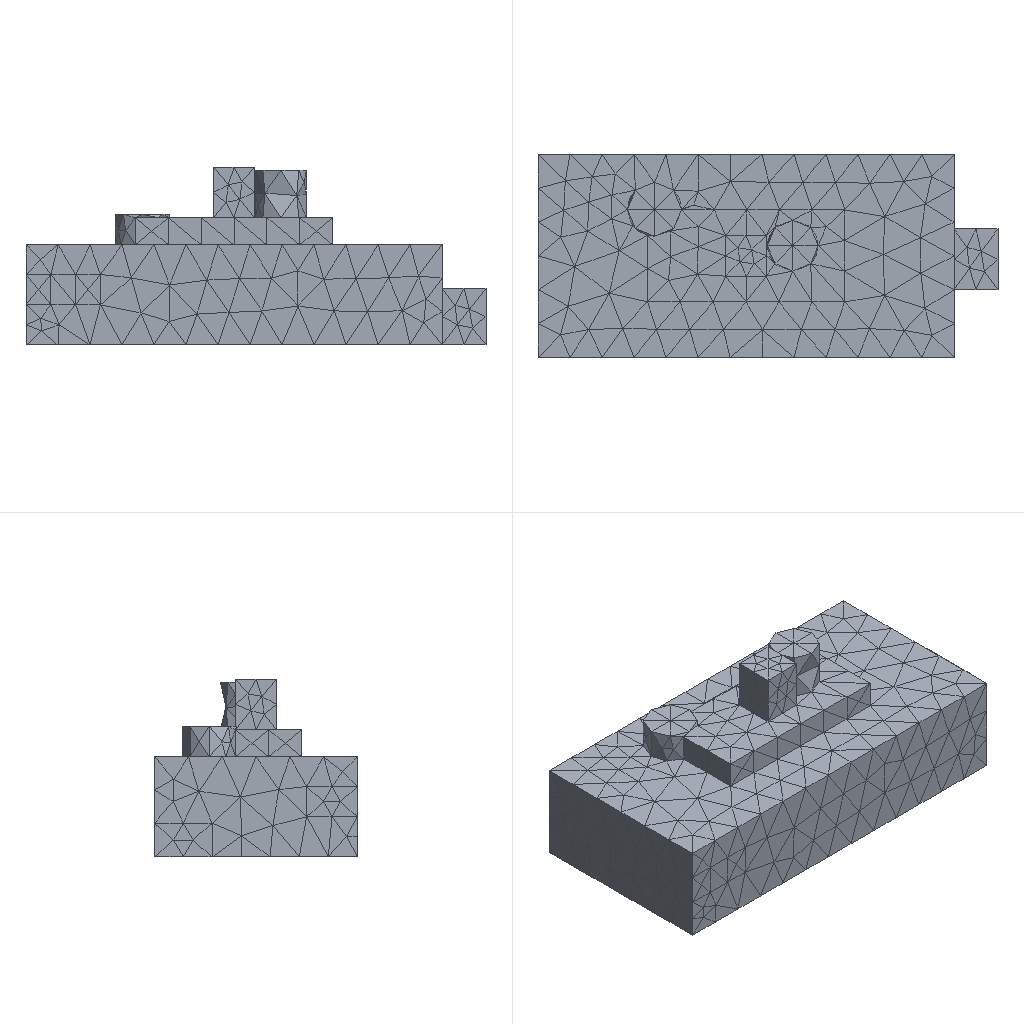Simulation study | ansys mapdl
Set-up summary:
category,name,step,type,value,unit,region
solver,ansys_mapdl
units,mm-N-s-tonne (MPa),,inferred,E=210000 density=
analysis,model,,static
mesh,nodes,,,4788
mesh,elements,,,2836
element_type,SOLID187,,,2836
material,mat 1,,E,210000
material,mat 1,,nu,0.3
load,,model,body load temp,,,all
load,,model,force,"1000 [dir=(0, 0, -1) n=237]",,node list
bc,,model,fixed,"[dofs=UX,UY,UZ n=5098]",,node list
Ansys APDL input file, long lists of numbers shortened:
/COM,ANSYS RELEASE 2026 R1           BUILD 26.1      UP20260202       09:08:46
/PREP7
/NOPR
/TITLE,2
ANTYPE, 0
*IF,_CDRDOFF,EQ,1,THEN     !if solid model was read in
_CDRDOFF=             !reset flag, numoffs already performed
*ELSE              !offset database for the following FE model
NUMOFF,NODE,     4788
NUMOFF,ELEM,     2836
NUMOFF,MAT ,        1
NUMOFF,TYPE,        1
*ENDIF
*SET,_RETURN ,  0.
*SET,_STATUS ,  0.
*SET,_UIQR   ,  237.
*SET,__FLOATPARAMETER__,  4788.
DOF,DELETE
ETBLOCK,        1,        1
(2i9,19a9)
        1      187        0        0        0        0        0        0        0        0        0        0        0        0        0        0        0        0        0        0        0
       -1
NBLOCK,6,SOLID,      4788,      4788
(3i9,6e21.13e3)
        1        0        0-6.0000000000000E+000-6.0000000000000E+000 5.2620000000000E+001
! (4787 more lines like these left out)
N,UNBL,LOC,       -1,
EBLOCK,19,SOLID,      2836,      2836
(19i10)
         1         1         1         1         0         0         0         0        10         0         1      1911      1912      1457      1913      2170      2171      2172      2173
! (5671 more lines like these left out)
        -1
MPTEMP,UNBL, 1, 1,  0.    ,
MPDATA,UNBL, 1,EX  ,       1, 1,  210000.000    ,
MPTEMP,UNBL, 1, 1,  0.    ,
MPDATA,UNBL, 1,NUXY,       1, 1, 0.3    ,
MPTEMP,UNBL, 1, 1,  0.    ,
MPDATA,UNBL, 1,PRXY,       1, 1, 0.3    ,
EXTOPT,ATTR,      0,      0,      0
EXTOPT,ESIZE,  0,  0.
EXTOPT,ACLEAR,      0
TREF,  0.
IRLF,  0
BFUNIF,TEMP,_TINY
ACEL,  0.    ,  0.    ,  0.
OMEGA,  0.    ,  0.    ,  0.
DOMEGA,  0.    ,  0.    ,  0.
CGLOC,  0.    ,  0.    ,  0.
CGOMEGA,  0.    ,  0.    ,  0.
DCGOMG,  0.    ,  0.    ,  0.
KUSE,     0
TIME,  0.
ALPHAD,  0.
BETAD,  0.
DMPRAT,  0.
DMPSTR,  0.
CRPLIM, 0.1    ,   0
CRPLIM,  0.    ,   1
NCNV,     0, 1.000000000E+12,     0,  0.    ,  0.
NEQIT,     0
ERESX,DEFA
DBLOCK,      5098
(i9,a6,2(pg16.9))
      315  UX    0.00000000      0.00000000
! (5097 more lines like these left out)
       -1
FBLOCK,       237
(i9,a6,2(pg16.9))
        1  FZ   -4.21940928      0.00000000
! (236 more lines like these left out)
       -1
/GO
FINISH
Results summary:
result,analysis_type_db,,,static,unstated
result,n_sets,,,1,unstated
result,load_steps[0].set,load_step=1,,1,unstated
result,load_steps[0].substep,load_step=1,,1,unstated
result,load_steps[0].time,load_step=1,,1,unstated
result,load_steps[0].freq,load_step=1,,1,unstated
result,load_steps[0].max_usum,load_step=1,,0.000492,unstated
result,load_steps[0].max_seqv,load_step=1,,4.902,unstated
result,load_steps[0].reaction_sum.FX,load_step=1,,-2.32571e-11,unstated
result,load_steps[0].reaction_sum.FY,load_step=1,,-8.33822e-12,unstated
result,load_steps[0].reaction_sum.FZ,load_step=1,,1000,unstated
result,load_steps[0].reaction_sum.MX,load_step=1,,0,unstated
result,load_steps[0].reaction_sum.MY,load_step=1,,0,unstated
result,load_steps[0].reaction_sum.MZ,load_step=1,,0,unstated
result,convergence,,,results present for all listed sets,unstated